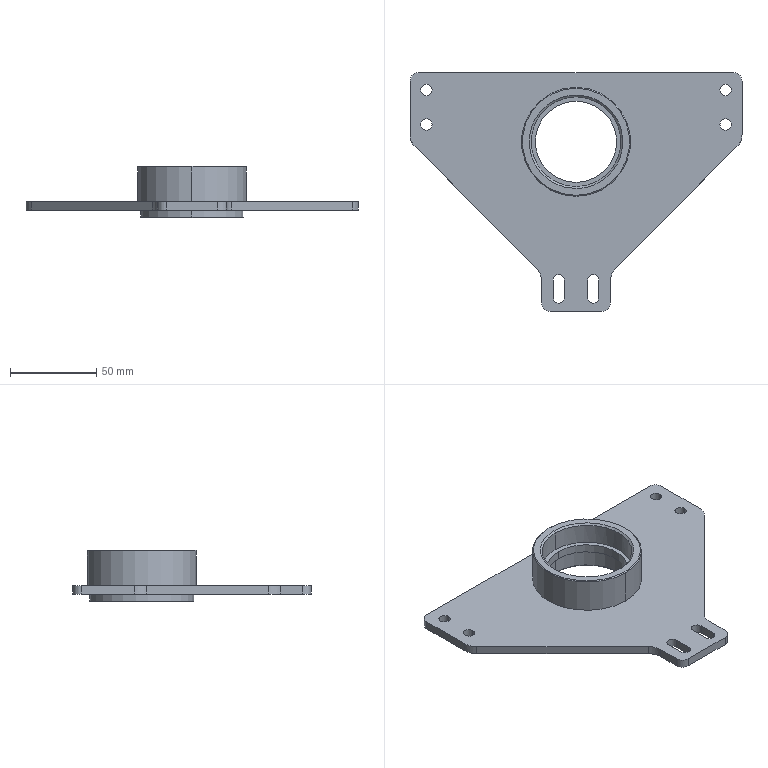Part | STEP file | 101000007788 | 2 solids | 59 faces | box 192 x 138 x 30 mm | volume 99773 mm3 | cylinder 32 | plane 19 | cone 8 | commonest cylinder face diameters 6.5 x12 10 x4 20 x4 52 x4 60 x4 47 x2